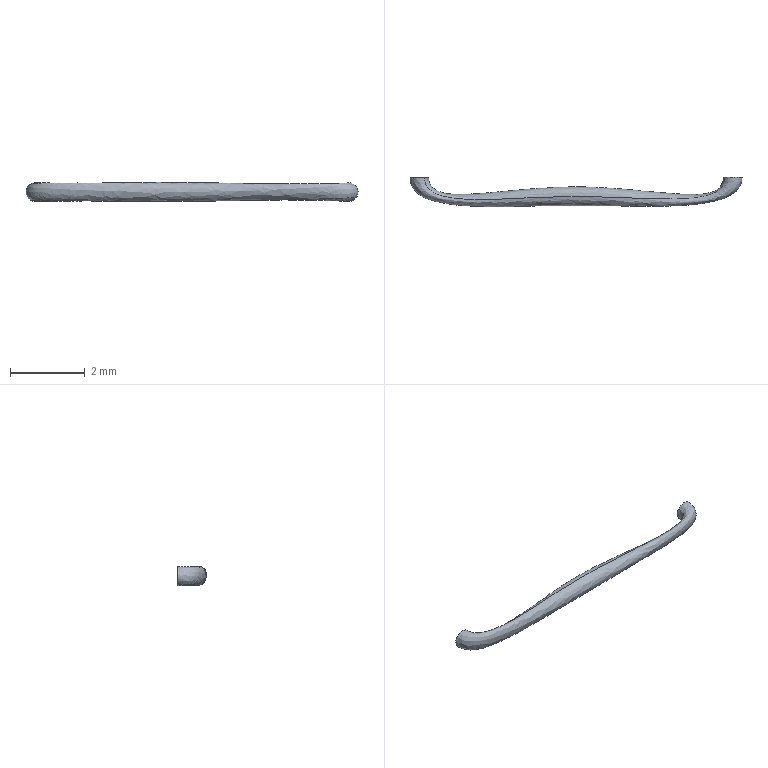Part | SolidWorks | features BaseBody 1 | 1 solid | 4 faces | box 8.882 x 0.784 x 0.5103 mm | volume 1.317 mm3 | plane 2 | spline 2
STEP:
#1=CARTESIAN_POINT('',(345.939,392.468,97.598));
#2=VERTEX_POINT('',#1);
#3=CARTESIAN_POINT('',(346.349,392.468,97.311));
#4=VERTEX_POINT('',#3);
#5=CARTESIAN_POINT('',(345.939,392.468,97.598));
#6=CARTESIAN_POINT('',(345.943,392.468,97.603));
#7=CARTESIAN_POINT('',(345.951,392.468,97.614));
#8=CARTESIAN_POINT('',(345.965,392.468,97.629));
#9=CARTESIAN_POINT('',(345.979,392.468,97.643));
#10=CARTESIAN_POINT('',(346.031,392.468,97.684));
#11=CARTESIAN_POINT('',(346.113,392.468,97.712));
#12=CARTESIAN_POINT('',(346.216,392.468,97.699));
#13=CARTESIAN_POINT('',(346.296,392.468,97.66));
#14=CARTESIAN_POINT('',(346.362,392.468,97.59));
#15=CARTESIAN_POINT('',(346.396,392.468,97.499));
#16=CARTESIAN_POINT('',(346.395,392.468,97.402));
#17=CARTESIAN_POINT('',(346.368,392.468,97.339));
#18=CARTESIAN_POINT('',(346.349,392.468,97.311));
#19=B_SPLINE_CURVE_WITH_KNOTS('',3,(#5,#6,#7,#8,#9,#10,#11,#12,#13,#14,#15,#16,#17,#18),.UNSPECIFIED.,.F.,.F.,(4,1,1,1,1,1,1,1,1,1,1,4),(0.,0.025,0.05,0.075,0.1,0.3,0.4,0.5,0.625,0.75,0.875,1.),.UNSPECIFIED.);
#20=EDGE_CURVE('',#2,#4,#19,.T.);
#21=ORIENTED_EDGE('',*,*,#20,.T.);
#22=CARTESIAN_POINT('',(346.349,392.468,97.311));
#23=CARTESIAN_POINT('',(346.33,392.468,97.284));
#24=CARTESIAN_POINT('',(346.28,392.468,97.237));
#25=CARTESIAN_POINT('',(346.189,392.468,97.203));
#26=CARTESIAN_POINT('',(346.092,392.468,97.203));
#27=CARTESIAN_POINT('',(346.004,392.468,97.241));
#28=CARTESIAN_POINT('',(345.94,392.468,97.303));
#29=CARTESIAN_POINT('',(345.892,392.468,97.395));
#30=CARTESIAN_POINT('',(345.889,392.468,97.482));
#31=CARTESIAN_POINT('',(345.911,392.468,97.544));
#32=CARTESIAN_POINT('',(345.918,392.468,97.563));
#33=CARTESIAN_POINT('',(345.928,392.468,97.58));
#34=CARTESIAN_POINT('',(345.935,392.468,97.592));
#35=CARTESIAN_POINT('',(345.939,392.468,97.598));
#36=B_SPLINE_CURVE_WITH_KNOTS('',3,(#22,#23,#24,#25,#26,#27,#28,#29,#30,#31,#32,#33,#34,#35),.UNSPECIFIED.,.F.,.F.,(4,1,1,1,1,1,1,1,1,1,1,4),(0.,0.125,0.25,0.375,0.5,0.6,0.7,0.9,0.925,0.95,0.975,1.),.UNSPECIFIED.);
#37=EDGE_CURVE('',#4,#2,#36,.T.);
#38=ORIENTED_EDGE('',*,*,#37,.T.);
#39=EDGE_LOOP('',(#21,#38));
#40=FACE_OUTER_BOUND('',#39,.T.);
#41=CARTESIAN_POINT('',(346.144,392.468,97.454));
#42=DIRECTION('',(0.0009599,-1.,0.));
#43=DIRECTION('',(0.,0.,-1.));
#44=AXIS2_PLACEMENT_3D('',#41,#42,#43);
#45=PLANE('',#44);
#46=ADVANCED_FACE('',(#40),#45,.F.);
#47=CARTESIAN_POINT('',(337.896,392.46,97.665));
#48=VERTEX_POINT('',#47);
#49=CARTESIAN_POINT('',(337.628,392.46,97.244));
#50=VERTEX_POINT('',#49);
#51=CARTESIAN_POINT('',(337.896,392.46,97.665));
#52=CARTESIAN_POINT('',(337.902,392.46,97.662));
#53=CARTESIAN_POINT('',(337.914,392.46,97.654));
#54=CARTESIAN_POINT('',(337.929,392.46,97.641));
#55=CARTESIAN_POINT('',(337.943,392.46,97.627));
#56=CARTESIAN_POINT('',(337.987,392.46,97.578));
#57=CARTESIAN_POINT('',(338.018,392.46,97.497));
#58=CARTESIAN_POINT('',(338.009,392.46,97.393));
#59=CARTESIAN_POINT('',(337.974,392.46,97.311));
#60=CARTESIAN_POINT('',(337.907,392.46,97.243));
#61=CARTESIAN_POINT('',(337.818,392.46,97.205));
#62=CARTESIAN_POINT('',(337.72,392.46,97.201));
#63=CARTESIAN_POINT('',(337.656,392.46,97.226));
#64=CARTESIAN_POINT('',(337.628,392.46,97.244));
#65=B_SPLINE_CURVE_WITH_KNOTS('',3,(#51,#52,#53,#54,#55,#56,#57,#58,#59,#60,#61,#62,#63,#64),.UNSPECIFIED.,.F.,.F.,(4,1,1,1,1,1,1,1,1,1,1,4),(0.,0.025,0.05,0.075,0.1,0.3,0.4,0.5,0.625,0.75,0.875,1.),.UNSPECIFIED.);
#66=EDGE_CURVE('',#48,#50,#65,.T.);
#67=ORIENTED_EDGE('',*,*,#66,.T.);
#68=CARTESIAN_POINT('',(337.628,392.46,97.244));
#69=CARTESIAN_POINT('',(337.6,392.46,97.262));
#70=CARTESIAN_POINT('',(337.551,392.46,97.309));
#71=CARTESIAN_POINT('',(337.512,392.46,97.399));
#72=CARTESIAN_POINT('',(337.509,392.46,97.496));
#73=CARTESIAN_POINT('',(337.543,392.46,97.586));
#74=CARTESIAN_POINT('',(337.602,392.46,97.652));
#75=CARTESIAN_POINT('',(337.692,392.46,97.704));
#76=CARTESIAN_POINT('',(337.779,392.46,97.71));
#77=CARTESIAN_POINT('',(337.842,392.46,97.692));
#78=CARTESIAN_POINT('',(337.861,392.46,97.685));
#79=CARTESIAN_POINT('',(337.879,392.46,97.676));
#80=CARTESIAN_POINT('',(337.891,392.46,97.669));
#81=CARTESIAN_POINT('',(337.896,392.46,97.665));
#82=B_SPLINE_CURVE_WITH_KNOTS('',3,(#68,#69,#70,#71,#72,#73,#74,#75,#76,#77,#78,#79,#80,#81),.UNSPECIFIED.,.F.,.F.,(4,1,1,1,1,1,1,1,1,1,1,4),(0.,0.125,0.25,0.375,0.5,0.6,0.7,0.9,0.925,0.95,0.975,1.),.UNSPECIFIED.);
#83=EDGE_CURVE('',#50,#48,#82,.T.);
#84=ORIENTED_EDGE('',*,*,#83,.T.);
#85=EDGE_LOOP('',(#67,#84));
#86=FACE_OUTER_BOUND('',#85,.T.);
#87=CARTESIAN_POINT('',(337.762,392.46,97.454));
#88=DIRECTION('',(0.0009599,-1.,0.));
#89=DIRECTION('',(0.,0.,-1.));
#90=AXIS2_PLACEMENT_3D('',#87,#88,#89);
#91=PLANE('',#90);
#92=ADVANCED_FACE('',(#86),#91,.F.);
#93=CARTESIAN_POINT('',(346.349,392.468,97.311));
#94=CARTESIAN_POINT('',(346.35,391.517,97.311));
#95=CARTESIAN_POINT('',(341.919,392.418,97.146));
#96=CARTESIAN_POINT('',(337.629,391.523,97.244));
#97=CARTESIAN_POINT('',(337.628,392.46,97.244));
#98=B_SPLINE_CURVE_WITH_KNOTS('',3,(#93,#94,#95,#96,#97),.UNSPECIFIED.,.F.,.F.,(4,1,4),(0.,0.5001,1.),.UNSPECIFIED.);
#99=EDGE_CURVE('',#4,#50,#98,.T.);
#100=ORIENTED_EDGE('',*,*,#99,.F.);
#101=ORIENTED_EDGE('',*,*,#20,.F.);
#102=CARTESIAN_POINT('',(337.896,392.46,97.665));
#103=CARTESIAN_POINT('',(337.897,391.575,97.665));
#104=CARTESIAN_POINT('',(341.99,392.332,97.792));
#105=CARTESIAN_POINT('',(345.94,391.597,97.598));
#106=CARTESIAN_POINT('',(345.939,392.468,97.598));
#107=B_SPLINE_CURVE_WITH_KNOTS('',3,(#102,#103,#104,#105,#106),.UNSPECIFIED.,.F.,.F.,(4,1,4),(0.,0.4999,1.),.UNSPECIFIED.);
#108=EDGE_CURVE('',#48,#2,#107,.T.);
#109=ORIENTED_EDGE('',*,*,#108,.F.);
#110=ORIENTED_EDGE('',*,*,#83,.F.);
#111=EDGE_LOOP('',(#100,#101,#109,#110));
#112=FACE_OUTER_BOUND('',#111,.T.);
#113=CARTESIAN_POINT('',(337.915,392.544,97.657));
#114=CARTESIAN_POINT('',(337.786,391.556,97.652));
#115=CARTESIAN_POINT('',(341.996,392.384,97.809));
#116=CARTESIAN_POINT('',(346.063,391.575,97.577));
#117=CARTESIAN_POINT('',(345.924,392.559,97.585));
#118=CARTESIAN_POINT('',(337.911,392.544,97.66));
#119=CARTESIAN_POINT('',(337.782,391.555,97.655));
#120=CARTESIAN_POINT('',(341.997,392.375,97.805));
#121=CARTESIAN_POINT('',(346.066,391.574,97.582));
#122=CARTESIAN_POINT('',(345.927,392.559,97.589));
#123=CARTESIAN_POINT('',(337.901,392.545,97.667));
#124=CARTESIAN_POINT('',(337.772,391.551,97.663));
#125=CARTESIAN_POINT('',(341.999,392.353,97.796));
#126=CARTESIAN_POINT('',(346.073,391.571,97.593));
#127=CARTESIAN_POINT('',(345.933,392.56,97.599));
#128=CARTESIAN_POINT('',(337.884,392.545,97.676));
#129=CARTESIAN_POINT('',(337.755,391.546,97.673));
#130=CARTESIAN_POINT('',(342.001,392.32,97.781));
#131=CARTESIAN_POINT('',(346.085,391.567,97.609));
#132=CARTESIAN_POINT('',(345.945,392.56,97.614));
#133=CARTESIAN_POINT('',(337.866,392.546,97.685));
#134=CARTESIAN_POINT('',(337.736,391.54,97.682));
#135=CARTESIAN_POINT('',(342.004,392.286,97.762));
#136=CARTESIAN_POINT('',(346.099,391.562,97.625));
#137=CARTESIAN_POINT('',(345.958,392.561,97.629));
#138=CARTESIAN_POINT('',(337.848,392.546,97.692));
#139=CARTESIAN_POINT('',(337.716,391.534,97.69));
#140=CARTESIAN_POINT('',(342.006,392.253,97.742));
#141=CARTESIAN_POINT('',(346.114,391.557,97.64));
#142=CARTESIAN_POINT('',(345.973,392.561,97.643));
#143=CARTESIAN_POINT('',(337.785,392.548,97.71));
#144=CARTESIAN_POINT('',(337.651,391.514,97.711));
#145=CARTESIAN_POINT('',(342.013,392.146,97.67));
#146=CARTESIAN_POINT('',(346.166,391.54,97.685));
#147=CARTESIAN_POINT('',(346.024,392.563,97.684));
#148=CARTESIAN_POINT('',(337.698,392.551,97.704));
#149=CARTESIAN_POINT('',(337.562,391.487,97.709));
#150=CARTESIAN_POINT('',(342.015,392.035,97.549));
#151=CARTESIAN_POINT('',(346.251,391.514,97.717));
#152=CARTESIAN_POINT('',(346.106,392.566,97.711));
#153=CARTESIAN_POINT('',(337.608,392.553,97.652));
#154=CARTESIAN_POINT('',(337.47,391.462,97.66));
#155=CARTESIAN_POINT('',(342.009,391.969,97.392));
#156=CARTESIAN_POINT('',(346.358,391.487,97.709));
#157=CARTESIAN_POINT('',(346.209,392.569,97.698));
#158=CARTESIAN_POINT('',(337.549,392.554,97.585));
#159=CARTESIAN_POINT('',(337.409,391.449,97.595));
#160=CARTESIAN_POINT('',(341.998,391.958,97.266));
#161=CARTESIAN_POINT('',(346.441,391.469,97.673));
#162=CARTESIAN_POINT('',(346.289,392.571,97.659));
#163=CARTESIAN_POINT('',(337.515,392.554,97.496));
#164=CARTESIAN_POINT('',(337.374,391.446,97.506));
#165=CARTESIAN_POINT('',(341.981,392.007,97.158));
#166=CARTESIAN_POINT('',(346.51,391.46,97.605));
#167=CARTESIAN_POINT('',(346.354,392.572,97.59));
#168=CARTESIAN_POINT('',(337.519,392.553,97.399));
#169=CARTESIAN_POINT('',(337.378,391.454,97.408));
#170=CARTESIAN_POINT('',(341.961,392.116,97.095));
#171=CARTESIAN_POINT('',(346.546,391.46,97.513));
#172=CARTESIAN_POINT('',(346.389,392.572,97.499));
#173=CARTESIAN_POINT('',(337.557,392.552,97.309));
#174=CARTESIAN_POINT('',(337.418,391.471,97.316));
#175=CARTESIAN_POINT('',(341.94,392.266,97.084));
#176=CARTESIAN_POINT('',(346.546,391.469,97.412));
#177=CARTESIAN_POINT('',(346.388,392.571,97.401));
#178=CARTESIAN_POINT('',(337.609,392.55,97.258));
#179=CARTESIAN_POINT('',(337.473,391.488,97.262));
#180=CARTESIAN_POINT('',(341.928,392.397,97.119));
#181=CARTESIAN_POINT('',(346.516,391.481,97.341));
#182=CARTESIAN_POINT('',(346.359,392.569,97.334));
#183=CARTESIAN_POINT('',(337.643,392.549,97.238));
#184=CARTESIAN_POINT('',(337.508,391.498,97.241));
#185=CARTESIAN_POINT('',(341.922,392.465,97.15));
#186=CARTESIAN_POINT('',(346.492,391.489,97.308));
#187=CARTESIAN_POINT('',(346.336,392.568,97.303));
#188=CARTESIAN_POINT('',(337.647,392.549,97.236));
#189=CARTESIAN_POINT('',(337.512,391.5,97.238));
#190=CARTESIAN_POINT('',(341.921,392.474,97.155));
#191=CARTESIAN_POINT('',(346.489,391.49,97.304));
#192=CARTESIAN_POINT('',(346.332,392.568,97.299));
#193=B_SPLINE_SURFACE_WITH_KNOTS('',3,3,((#113,#114,#115,#116,#117),(#118,#119,#120,#121,#122),(#123,#124,#125,#126,#127),(#128,#129,#130,#131,#132),(#133,#134,#135,#136,#137),(#138,#139,#140,#141,#142),(#143,#144,#145,#146,#147),(#148,#149,#150,#151,#152),(#153,#154,#155,#156,#157),(#158,#159,#160,#161,#162),(#163,#164,#165,#166,#167),(#168,#169,#170,#171,#172),(#173,#174,#175,#176,#177),(#178,#179,#180,#181,#182),(#183,#184,#185,#186,#187),(#188,#189,#190,#191,#192)),.UNSPECIFIED.,.F.,.F.,.F.,(4,1,1,1,1,1,1,1,1,1,1,1,1,4),(4,1,4),(-0.009538,0.,0.0125,0.025,0.0375,0.05,0.15,0.2,0.25,0.3125,0.375,0.4375,0.5,0.5095),(-0.01521,0.4999,1.017),.UNSPECIFIED.);
#194=ADVANCED_FACE('',(#112),#193,.T.);
#195=ORIENTED_EDGE('',*,*,#66,.F.);
#196=ORIENTED_EDGE('',*,*,#108,.T.);
#197=ORIENTED_EDGE('',*,*,#37,.F.);
#198=ORIENTED_EDGE('',*,*,#99,.T.);
#199=EDGE_LOOP('',(#195,#196,#197,#198));
#200=FACE_OUTER_BOUND('',#199,.T.);
#201=CARTESIAN_POINT('',(337.621,392.55,97.252));
#202=CARTESIAN_POINT('',(337.485,391.492,97.256));
#203=CARTESIAN_POINT('',(341.926,392.42,97.131));
#204=CARTESIAN_POINT('',(346.507,391.484,97.331));
#205=CARTESIAN_POINT('',(346.35,392.569,97.324));
#206=CARTESIAN_POINT('',(337.625,392.55,97.249));
#207=CARTESIAN_POINT('',(337.49,391.493,97.253));
#208=CARTESIAN_POINT('',(341.925,392.429,97.135));
#209=CARTESIAN_POINT('',(346.504,391.485,97.326));
#210=CARTESIAN_POINT('',(346.347,392.569,97.32));
#211=CARTESIAN_POINT('',(337.657,392.549,97.227));
#212=CARTESIAN_POINT('',(337.523,391.503,97.229));
#213=CARTESIAN_POINT('',(341.919,392.498,97.163));
#214=CARTESIAN_POINT('',(346.483,391.492,97.292));
#215=CARTESIAN_POINT('',(346.326,392.568,97.287));
#216=CARTESIAN_POINT('',(337.726,392.547,97.201));
#217=CARTESIAN_POINT('',(337.594,391.523,97.2));
#218=CARTESIAN_POINT('',(341.911,392.623,97.237));
#219=CARTESIAN_POINT('',(346.427,391.509,97.237));
#220=CARTESIAN_POINT('',(346.273,392.566,97.237));
#221=CARTESIAN_POINT('',(337.823,392.544,97.205));
#222=CARTESIAN_POINT('',(337.694,391.552,97.2));
#223=CARTESIAN_POINT('',(341.907,392.753,97.371));
#224=CARTESIAN_POINT('',(346.333,391.536,97.197));
#225=CARTESIAN_POINT('',(346.182,392.563,97.203));
#226=CARTESIAN_POINT('',(337.913,392.541,97.243));
#227=CARTESIAN_POINT('',(337.787,391.577,97.235));
#228=CARTESIAN_POINT('',(341.911,392.834,97.518));
#229=CARTESIAN_POINT('',(346.233,391.562,97.193));
#230=CARTESIAN_POINT('',(346.084,392.56,97.204));
#231=CARTESIAN_POINT('',(337.98,392.54,97.312));
#232=CARTESIAN_POINT('',(337.855,391.593,97.301));
#233=CARTESIAN_POINT('',(341.922,392.852,97.656));
#234=CARTESIAN_POINT('',(346.141,391.582,97.227));
#235=CARTESIAN_POINT('',(345.997,392.558,97.242));
#236=CARTESIAN_POINT('',(338.015,392.54,97.394));
#237=CARTESIAN_POINT('',(337.891,391.599,97.382));
#238=CARTESIAN_POINT('',(341.938,392.81,97.76));
#239=CARTESIAN_POINT('',(346.075,391.594,97.288));
#240=CARTESIAN_POINT('',(345.933,392.557,97.304));
#241=CARTESIAN_POINT('',(338.023,392.54,97.497));
#242=CARTESIAN_POINT('',(337.899,391.597,97.487));
#243=CARTESIAN_POINT('',(341.958,392.709,97.844));
#244=CARTESIAN_POINT('',(346.025,391.599,97.381));
#245=CARTESIAN_POINT('',(345.885,392.556,97.396));
#246=CARTESIAN_POINT('',(337.992,392.541,97.578));
#247=CARTESIAN_POINT('',(337.867,391.583,97.569));
#248=CARTESIAN_POINT('',(341.976,392.577,97.858));
#249=CARTESIAN_POINT('',(346.021,391.594,97.47));
#250=CARTESIAN_POINT('',(345.883,392.557,97.483));
#251=CARTESIAN_POINT('',(337.949,392.543,97.627));
#252=CARTESIAN_POINT('',(337.821,391.568,97.621));
#253=CARTESIAN_POINT('',(341.988,392.463,97.834));
#254=CARTESIAN_POINT('',(346.043,391.583,97.535));
#255=CARTESIAN_POINT('',(345.904,392.558,97.545));
#256=CARTESIAN_POINT('',(337.935,392.543,97.641));
#257=CARTESIAN_POINT('',(337.807,391.563,97.636));
#258=CARTESIAN_POINT('',(341.992,392.428,97.824));
#259=CARTESIAN_POINT('',(346.051,391.58,97.554));
#260=CARTESIAN_POINT('',(345.912,392.559,97.563));
#261=CARTESIAN_POINT('',(337.919,392.544,97.654));
#262=CARTESIAN_POINT('',(337.79,391.558,97.649));
#263=CARTESIAN_POINT('',(341.995,392.393,97.812));
#264=CARTESIAN_POINT('',(346.061,391.576,97.573));
#265=CARTESIAN_POINT('',(345.921,392.559,97.581));
#266=CARTESIAN_POINT('',(337.904,392.544,97.665));
#267=CARTESIAN_POINT('',(337.774,391.552,97.661));
#268=CARTESIAN_POINT('',(341.998,392.359,97.799));
#269=CARTESIAN_POINT('',(346.071,391.572,97.59));
#270=CARTESIAN_POINT('',(345.931,392.56,97.597));
#271=CARTESIAN_POINT('',(337.893,392.545,97.671));
#272=CARTESIAN_POINT('',(337.764,391.549,97.667));
#273=CARTESIAN_POINT('',(342.,392.338,97.789));
#274=CARTESIAN_POINT('',(346.079,391.569,97.6));
#275=CARTESIAN_POINT('',(345.939,392.56,97.606));
#276=CARTESIAN_POINT('',(337.889,392.545,97.674));
#277=CARTESIAN_POINT('',(337.759,391.547,97.67));
#278=CARTESIAN_POINT('',(342.001,392.329,97.785));
#279=CARTESIAN_POINT('',(346.082,391.568,97.604));
#280=CARTESIAN_POINT('',(345.942,392.56,97.61));
#281=B_SPLINE_SURFACE_WITH_KNOTS('',3,3,((#201,#202,#203,#204,#205),(#206,#207,#208,#209,#210),(#211,#212,#213,#214,#215),(#216,#217,#218,#219,#220),(#221,#222,#223,#224,#225),(#226,#227,#228,#229,#230),(#231,#232,#233,#234,#235),(#236,#237,#238,#239,#240),(#241,#242,#243,#244,#245),(#246,#247,#248,#249,#250),(#251,#252,#253,#254,#255),(#256,#257,#258,#259,#260),(#261,#262,#263,#264,#265),(#266,#267,#268,#269,#270),(#271,#272,#273,#274,#275),(#276,#277,#278,#279,#280)),.UNSPECIFIED.,.F.,.F.,.F.,(4,1,1,1,1,1,1,1,1,1,1,1,1,4),(4,1,4),(0.4905,0.5,0.5625,0.625,0.6875,0.75,0.8,0.85,0.95,0.9625,0.975,0.9875,1.,1.01),(-0.01521,0.4999,1.017),.UNSPECIFIED.);
#282=ADVANCED_FACE('',(#200),#281,.T.);
#283=CLOSED_SHELL('',(#46,#92,#194,#282));
#284=MANIFOLD_SOLID_BREP('',#283);
#285=CARTESIAN_POINT('',(0.,0.,0.));
#286=DIRECTION('',(0.,0.,1.));
#287=DIRECTION('',(1.,0.,0.));
#288=AXIS2_PLACEMENT_3D('',#285,#286,#287);
#289=(LENGTH_UNIT()NAMED_UNIT(*)SI_UNIT(.MILLI.,.METRE.));
#290=UNCERTAINTY_MEASURE_WITH_UNIT(LENGTH_MEASURE(0.00001),#289,'','');
#291=(NAMED_UNIT(*)PLANE_ANGLE_UNIT()SI_UNIT($,.RADIAN.));
#292=(NAMED_UNIT(*)SI_UNIT($,.STERADIAN.)SOLID_ANGLE_UNIT());
#293=(GEOMETRIC_REPRESENTATION_CONTEXT(3)GLOBAL_UNCERTAINTY_ASSIGNED_CONTEXT((#290))GLOBAL_UNIT_ASSIGNED_CONTEXT((#289,#291,#292))REPRESENTATION_CONTEXT('',''));
#294=ADVANCED_BREP_SHAPE_REPRESENTATION('',(#284,#288),#293);